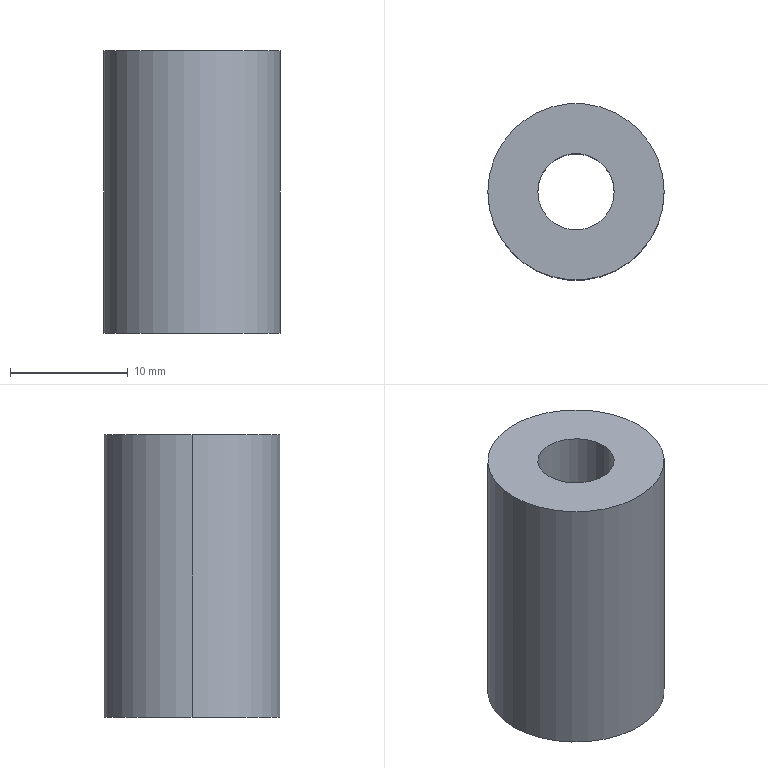Part | STEP file | track support post | 1 solid | 6 faces | box 15 x 15 x 24 mm | volume 3445 mm3 | cylinder 4 | plane 2 | commonest cylinder face diameters 6.5 x2 15 x2
STEP:
#1=CARTESIAN_POINT('',(0.,0.,0.));
#2=DIRECTION('',(0.,0.,1.));
#3=DIRECTION('',(1.,0.,0.));
#4=AXIS2_PLACEMENT_3D('',#1,#2,#3);
#5=CARTESIAN_POINT('',(3.25,0.,0.));
#6=VERTEX_POINT('',#5);
#7=CARTESIAN_POINT('',(3.25,0.,24.));
#8=VERTEX_POINT('',#7);
#9=CARTESIAN_POINT('',(3.25,0.,0.));
#10=DIRECTION('',(0.,0.,1.));
#11=VECTOR('',#10,1.);
#12=LINE('',#9,#11);
#13=CARTESIAN_POINT('',(0.,0.,0.));
#14=DIRECTION('',(0.,0.,1.));
#15=DIRECTION('',(1.,0.,0.));
#16=AXIS2_PLACEMENT_3D('',#13,#14,#15);
#17=CYLINDRICAL_SURFACE('',#16,3.25);
#18=CARTESIAN_POINT('',(6.283,0.));
#19=DIRECTION('',(0.,1.));
#20=VECTOR('',#19,1.);
#21=LINE('',#18,#20);
#22=(GEOMETRIC_REPRESENTATION_CONTEXT(2)PARAMETRIC_REPRESENTATION_CONTEXT()REPRESENTATION_CONTEXT('',''));
#23=DEFINITIONAL_REPRESENTATION('',(#21),#22);
#24=PCURVE('',#17,#23);
#25=CARTESIAN_POINT('',(0.,0.,0.));
#26=DIRECTION('',(0.,0.,1.));
#27=DIRECTION('',(1.,0.,0.));
#28=AXIS2_PLACEMENT_3D('',#25,#26,#27);
#29=CYLINDRICAL_SURFACE('',#28,3.25);
#30=CARTESIAN_POINT('',(0.,0.));
#31=DIRECTION('',(0.,1.));
#32=VECTOR('',#31,1.);
#33=LINE('',#30,#32);
#34=(GEOMETRIC_REPRESENTATION_CONTEXT(2)PARAMETRIC_REPRESENTATION_CONTEXT()REPRESENTATION_CONTEXT('',''));
#35=DEFINITIONAL_REPRESENTATION('',(#33),#34);
#36=PCURVE('',#29,#35);
#37=SURFACE_CURVE('',#12,(#24,#36),.PCURVE_S1.);
#38=EDGE_CURVE('',#6,#8,#37,.T.);
#39=ORIENTED_EDGE('',*,*,#38,.T.);
#40=CARTESIAN_POINT('',(-3.25,0.,24.));
#41=VERTEX_POINT('',#40);
#42=CARTESIAN_POINT('',(0.,0.,24.));
#43=DIRECTION('',(0.,0.,1.));
#44=DIRECTION('',(1.,0.,0.));
#45=AXIS2_PLACEMENT_3D('',#42,#43,#44);
#46=CIRCLE('',#45,3.25);
#47=CARTESIAN_POINT('',(0.,24.));
#48=DIRECTION('',(1.,0.));
#49=VECTOR('',#48,1.);
#50=LINE('',#47,#49);
#51=(GEOMETRIC_REPRESENTATION_CONTEXT(2)PARAMETRIC_REPRESENTATION_CONTEXT()REPRESENTATION_CONTEXT('',''));
#52=DEFINITIONAL_REPRESENTATION('',(#50),#51);
#53=PCURVE('',#17,#52);
#54=CARTESIAN_POINT('',(0.,0.,24.));
#55=DIRECTION('',(0.,0.,1.));
#56=DIRECTION('',(1.,0.,0.));
#57=AXIS2_PLACEMENT_3D('',#54,#55,#56);
#58=PLANE('',#57);
#59=CARTESIAN_POINT('',(0.,0.));
#60=DIRECTION('',(1.,0.));
#61=AXIS2_PLACEMENT_2D('',#59,#60);
#62=CIRCLE('',#61,3.25);
#63=(GEOMETRIC_REPRESENTATION_CONTEXT(2)PARAMETRIC_REPRESENTATION_CONTEXT()REPRESENTATION_CONTEXT('',''));
#64=DEFINITIONAL_REPRESENTATION('',(#62),#63);
#65=PCURVE('',#58,#64);
#66=SURFACE_CURVE('',#46,(#53,#65),.PCURVE_S1.);
#67=EDGE_CURVE('',#41,#8,#66,.T.);
#68=ORIENTED_EDGE('',*,*,#67,.F.);
#69=CARTESIAN_POINT('',(-3.25,0.,0.));
#70=VERTEX_POINT('',#69);
#71=CARTESIAN_POINT('',(-3.25,0.,0.));
#72=DIRECTION('',(0.,0.,1.));
#73=VECTOR('',#72,1.);
#74=LINE('',#71,#73);
#75=CARTESIAN_POINT('',(3.142,0.));
#76=DIRECTION('',(0.,1.));
#77=VECTOR('',#76,1.);
#78=LINE('',#75,#77);
#79=(GEOMETRIC_REPRESENTATION_CONTEXT(2)PARAMETRIC_REPRESENTATION_CONTEXT()REPRESENTATION_CONTEXT('',''));
#80=DEFINITIONAL_REPRESENTATION('',(#78),#79);
#81=PCURVE('',#17,#80);
#82=CARTESIAN_POINT('',(3.142,0.));
#83=DIRECTION('',(0.,1.));
#84=VECTOR('',#83,1.);
#85=LINE('',#82,#84);
#86=(GEOMETRIC_REPRESENTATION_CONTEXT(2)PARAMETRIC_REPRESENTATION_CONTEXT()REPRESENTATION_CONTEXT('',''));
#87=DEFINITIONAL_REPRESENTATION('',(#85),#86);
#88=PCURVE('',#29,#87);
#89=SURFACE_CURVE('',#74,(#81,#88),.PCURVE_S1.);
#90=EDGE_CURVE('',#70,#41,#89,.T.);
#91=ORIENTED_EDGE('',*,*,#90,.F.);
#92=CARTESIAN_POINT('',(0.,0.,0.));
#93=DIRECTION('',(0.,0.,1.));
#94=DIRECTION('',(1.,0.,0.));
#95=AXIS2_PLACEMENT_3D('',#92,#93,#94);
#96=CIRCLE('',#95,3.25);
#97=CARTESIAN_POINT('',(0.,0.));
#98=DIRECTION('',(1.,0.));
#99=VECTOR('',#98,1.);
#100=LINE('',#97,#99);
#101=(GEOMETRIC_REPRESENTATION_CONTEXT(2)PARAMETRIC_REPRESENTATION_CONTEXT()REPRESENTATION_CONTEXT('',''));
#102=DEFINITIONAL_REPRESENTATION('',(#100),#101);
#103=PCURVE('',#17,#102);
#104=CARTESIAN_POINT('',(0.,0.,0.));
#105=DIRECTION('',(0.,0.,1.));
#106=DIRECTION('',(1.,0.,0.));
#107=AXIS2_PLACEMENT_3D('',#104,#105,#106);
#108=PLANE('',#107);
#109=CARTESIAN_POINT('',(0.,0.));
#110=DIRECTION('',(1.,0.));
#111=AXIS2_PLACEMENT_2D('',#109,#110);
#112=CIRCLE('',#111,3.25);
#113=(GEOMETRIC_REPRESENTATION_CONTEXT(2)PARAMETRIC_REPRESENTATION_CONTEXT()REPRESENTATION_CONTEXT('',''));
#114=DEFINITIONAL_REPRESENTATION('',(#112),#113);
#115=PCURVE('',#108,#114);
#116=SURFACE_CURVE('',#96,(#103,#115),.PCURVE_S1.);
#117=EDGE_CURVE('',#70,#6,#116,.T.);
#118=ORIENTED_EDGE('',*,*,#117,.T.);
#119=EDGE_LOOP('',(#39,#68,#91,#118));
#120=FACE_BOUND('',#119,.F.);
#121=ADVANCED_FACE('',(#120),#17,.F.);
#122=CARTESIAN_POINT('',(7.5,0.,24.));
#123=VERTEX_POINT('',#122);
#124=CARTESIAN_POINT('',(-7.5,0.,24.));
#125=VERTEX_POINT('',#124);
#126=CARTESIAN_POINT('',(0.,0.,24.));
#127=DIRECTION('',(0.,0.,1.));
#128=DIRECTION('',(1.,0.,0.));
#129=AXIS2_PLACEMENT_3D('',#126,#127,#128);
#130=CIRCLE('',#129,7.5);
#131=CARTESIAN_POINT('',(0.,0.,24.));
#132=DIRECTION('',(0.,0.,-1.));
#133=DIRECTION('',(-1.,0.,0.));
#134=AXIS2_PLACEMENT_3D('',#131,#132,#133);
#135=CYLINDRICAL_SURFACE('',#134,7.5);
#136=CARTESIAN_POINT('',(3.142,0.));
#137=DIRECTION('',(-1.,0.));
#138=VECTOR('',#137,1.);
#139=LINE('',#136,#138);
#140=(GEOMETRIC_REPRESENTATION_CONTEXT(2)PARAMETRIC_REPRESENTATION_CONTEXT()REPRESENTATION_CONTEXT('',''));
#141=DEFINITIONAL_REPRESENTATION('',(#139),#140);
#142=PCURVE('',#135,#141);
#143=CARTESIAN_POINT('',(0.,0.));
#144=DIRECTION('',(1.,0.));
#145=AXIS2_PLACEMENT_2D('',#143,#144);
#146=CIRCLE('',#145,7.5);
#147=(GEOMETRIC_REPRESENTATION_CONTEXT(2)PARAMETRIC_REPRESENTATION_CONTEXT()REPRESENTATION_CONTEXT('',''));
#148=DEFINITIONAL_REPRESENTATION('',(#146),#147);
#149=PCURVE('',#58,#148);
#150=SURFACE_CURVE('',#130,(#142,#149),.PCURVE_S1.);
#151=EDGE_CURVE('',#123,#125,#150,.T.);
#152=ORIENTED_EDGE('',*,*,#151,.F.);
#153=CARTESIAN_POINT('',(7.5,0.,0.));
#154=VERTEX_POINT('',#153);
#155=CARTESIAN_POINT('',(7.5,0.,24.));
#156=DIRECTION('',(0.,0.,-1.));
#157=VECTOR('',#156,1.);
#158=LINE('',#155,#157);
#159=CARTESIAN_POINT('',(3.142,0.));
#160=DIRECTION('',(0.,1.));
#161=VECTOR('',#160,1.);
#162=LINE('',#159,#161);
#163=(GEOMETRIC_REPRESENTATION_CONTEXT(2)PARAMETRIC_REPRESENTATION_CONTEXT()REPRESENTATION_CONTEXT('',''));
#164=DEFINITIONAL_REPRESENTATION('',(#162),#163);
#165=PCURVE('',#135,#164);
#166=CARTESIAN_POINT('',(0.,0.,24.));
#167=DIRECTION('',(0.,0.,-1.));
#168=DIRECTION('',(-1.,0.,0.));
#169=AXIS2_PLACEMENT_3D('',#166,#167,#168);
#170=CYLINDRICAL_SURFACE('',#169,7.5);
#171=CARTESIAN_POINT('',(3.142,0.));
#172=DIRECTION('',(0.,1.));
#173=VECTOR('',#172,1.);
#174=LINE('',#171,#173);
#175=(GEOMETRIC_REPRESENTATION_CONTEXT(2)PARAMETRIC_REPRESENTATION_CONTEXT()REPRESENTATION_CONTEXT('',''));
#176=DEFINITIONAL_REPRESENTATION('',(#174),#175);
#177=PCURVE('',#170,#176);
#178=SURFACE_CURVE('',#158,(#165,#177),.PCURVE_S1.);
#179=EDGE_CURVE('',#123,#154,#178,.T.);
#180=ORIENTED_EDGE('',*,*,#179,.T.);
#181=CARTESIAN_POINT('',(-7.5,0.,0.));
#182=VERTEX_POINT('',#181);
#183=CARTESIAN_POINT('',(0.,0.,0.));
#184=DIRECTION('',(0.,0.,1.));
#185=DIRECTION('',(1.,0.,0.));
#186=AXIS2_PLACEMENT_3D('',#183,#184,#185);
#187=CIRCLE('',#186,7.5);
#188=CARTESIAN_POINT('',(3.142,24.));
#189=DIRECTION('',(-1.,0.));
#190=VECTOR('',#189,1.);
#191=LINE('',#188,#190);
#192=(GEOMETRIC_REPRESENTATION_CONTEXT(2)PARAMETRIC_REPRESENTATION_CONTEXT()REPRESENTATION_CONTEXT('',''));
#193=DEFINITIONAL_REPRESENTATION('',(#191),#192);
#194=PCURVE('',#135,#193);
#195=CARTESIAN_POINT('',(0.,0.));
#196=DIRECTION('',(1.,0.));
#197=AXIS2_PLACEMENT_2D('',#195,#196);
#198=CIRCLE('',#197,7.5);
#199=(GEOMETRIC_REPRESENTATION_CONTEXT(2)PARAMETRIC_REPRESENTATION_CONTEXT()REPRESENTATION_CONTEXT('',''));
#200=DEFINITIONAL_REPRESENTATION('',(#198),#199);
#201=PCURVE('',#108,#200);
#202=SURFACE_CURVE('',#187,(#194,#201),.PCURVE_S1.);
#203=EDGE_CURVE('',#154,#182,#202,.T.);
#204=ORIENTED_EDGE('',*,*,#203,.T.);
#205=CARTESIAN_POINT('',(-7.5,0.,24.));
#206=DIRECTION('',(0.,0.,-1.));
#207=VECTOR('',#206,1.);
#208=LINE('',#205,#207);
#209=CARTESIAN_POINT('',(0.,0.));
#210=DIRECTION('',(0.,1.));
#211=VECTOR('',#210,1.);
#212=LINE('',#209,#211);
#213=(GEOMETRIC_REPRESENTATION_CONTEXT(2)PARAMETRIC_REPRESENTATION_CONTEXT()REPRESENTATION_CONTEXT('',''));
#214=DEFINITIONAL_REPRESENTATION('',(#212),#213);
#215=PCURVE('',#135,#214);
#216=CARTESIAN_POINT('',(6.283,0.));
#217=DIRECTION('',(0.,1.));
#218=VECTOR('',#217,1.);
#219=LINE('',#216,#218);
#220=(GEOMETRIC_REPRESENTATION_CONTEXT(2)PARAMETRIC_REPRESENTATION_CONTEXT()REPRESENTATION_CONTEXT('',''));
#221=DEFINITIONAL_REPRESENTATION('',(#219),#220);
#222=PCURVE('',#170,#221);
#223=SURFACE_CURVE('',#208,(#215,#222),.PCURVE_S1.);
#224=EDGE_CURVE('',#125,#182,#223,.T.);
#225=ORIENTED_EDGE('',*,*,#224,.F.);
#226=EDGE_LOOP('',(#152,#180,#204,#225));
#227=FACE_BOUND('',#226,.T.);
#228=ADVANCED_FACE('',(#227),#135,.T.);
#229=ORIENTED_EDGE('',*,*,#179,.F.);
#230=CARTESIAN_POINT('',(0.,0.,24.));
#231=DIRECTION('',(0.,0.,1.));
#232=DIRECTION('',(1.,0.,0.));
#233=AXIS2_PLACEMENT_3D('',#230,#231,#232);
#234=CIRCLE('',#233,7.5);
#235=CARTESIAN_POINT('',(9.425,0.));
#236=DIRECTION('',(-1.,0.));
#237=VECTOR('',#236,1.);
#238=LINE('',#235,#237);
#239=(GEOMETRIC_REPRESENTATION_CONTEXT(2)PARAMETRIC_REPRESENTATION_CONTEXT()REPRESENTATION_CONTEXT('',''));
#240=DEFINITIONAL_REPRESENTATION('',(#238),#239);
#241=PCURVE('',#170,#240);
#242=CARTESIAN_POINT('',(0.,0.));
#243=DIRECTION('',(1.,0.));
#244=AXIS2_PLACEMENT_2D('',#242,#243);
#245=CIRCLE('',#244,7.5);
#246=(GEOMETRIC_REPRESENTATION_CONTEXT(2)PARAMETRIC_REPRESENTATION_CONTEXT()REPRESENTATION_CONTEXT('',''));
#247=DEFINITIONAL_REPRESENTATION('',(#245),#246);
#248=PCURVE('',#58,#247);
#249=SURFACE_CURVE('',#234,(#241,#248),.PCURVE_S1.);
#250=EDGE_CURVE('',#125,#123,#249,.T.);
#251=ORIENTED_EDGE('',*,*,#250,.F.);
#252=ORIENTED_EDGE('',*,*,#224,.T.);
#253=CARTESIAN_POINT('',(0.,0.,0.));
#254=DIRECTION('',(0.,0.,1.));
#255=DIRECTION('',(1.,0.,0.));
#256=AXIS2_PLACEMENT_3D('',#253,#254,#255);
#257=CIRCLE('',#256,7.5);
#258=CARTESIAN_POINT('',(9.425,24.));
#259=DIRECTION('',(-1.,0.));
#260=VECTOR('',#259,1.);
#261=LINE('',#258,#260);
#262=(GEOMETRIC_REPRESENTATION_CONTEXT(2)PARAMETRIC_REPRESENTATION_CONTEXT()REPRESENTATION_CONTEXT('',''));
#263=DEFINITIONAL_REPRESENTATION('',(#261),#262);
#264=PCURVE('',#170,#263);
#265=CARTESIAN_POINT('',(0.,0.));
#266=DIRECTION('',(1.,0.));
#267=AXIS2_PLACEMENT_2D('',#265,#266);
#268=CIRCLE('',#267,7.5);
#269=(GEOMETRIC_REPRESENTATION_CONTEXT(2)PARAMETRIC_REPRESENTATION_CONTEXT()REPRESENTATION_CONTEXT('',''));
#270=DEFINITIONAL_REPRESENTATION('',(#268),#269);
#271=PCURVE('',#108,#270);
#272=SURFACE_CURVE('',#257,(#264,#271),.PCURVE_S1.);
#273=EDGE_CURVE('',#182,#154,#272,.T.);
#274=ORIENTED_EDGE('',*,*,#273,.T.);
#275=EDGE_LOOP('',(#229,#251,#252,#274));
#276=FACE_BOUND('',#275,.T.);
#277=ADVANCED_FACE('',(#276),#170,.T.);
#278=CARTESIAN_POINT('',(0.,0.,24.));
#279=DIRECTION('',(0.,0.,1.));
#280=DIRECTION('',(1.,0.,0.));
#281=AXIS2_PLACEMENT_3D('',#278,#279,#280);
#282=CIRCLE('',#281,3.25);
#283=CARTESIAN_POINT('',(0.,0.));
#284=DIRECTION('',(1.,0.));
#285=AXIS2_PLACEMENT_2D('',#283,#284);
#286=CIRCLE('',#285,3.25);
#287=(GEOMETRIC_REPRESENTATION_CONTEXT(2)PARAMETRIC_REPRESENTATION_CONTEXT()REPRESENTATION_CONTEXT('',''));
#288=DEFINITIONAL_REPRESENTATION('',(#286),#287);
#289=PCURVE('',#58,#288);
#290=CARTESIAN_POINT('',(0.,24.));
#291=DIRECTION('',(1.,0.));
#292=VECTOR('',#291,1.);
#293=LINE('',#290,#292);
#294=(GEOMETRIC_REPRESENTATION_CONTEXT(2)PARAMETRIC_REPRESENTATION_CONTEXT()REPRESENTATION_CONTEXT('',''));
#295=DEFINITIONAL_REPRESENTATION('',(#293),#294);
#296=PCURVE('',#29,#295);
#297=SURFACE_CURVE('',#282,(#289,#296),.PCURVE_S1.);
#298=EDGE_CURVE('',#8,#41,#297,.T.);
#299=ORIENTED_EDGE('',*,*,#298,.F.);
#300=ORIENTED_EDGE('',*,*,#67,.F.);
#301=EDGE_LOOP('',(#299,#300));
#302=FACE_BOUND('',#301,.T.);
#303=ORIENTED_EDGE('',*,*,#250,.T.);
#304=ORIENTED_EDGE('',*,*,#151,.T.);
#305=EDGE_LOOP('',(#303,#304));
#306=FACE_BOUND('',#305,.T.);
#307=ADVANCED_FACE('',(#302,#306),#58,.T.);
#308=CARTESIAN_POINT('',(0.,0.,0.));
#309=DIRECTION('',(0.,0.,1.));
#310=DIRECTION('',(1.,0.,0.));
#311=AXIS2_PLACEMENT_3D('',#308,#309,#310);
#312=CIRCLE('',#311,3.25);
#313=CARTESIAN_POINT('',(0.,0.));
#314=DIRECTION('',(1.,0.));
#315=AXIS2_PLACEMENT_2D('',#313,#314);
#316=CIRCLE('',#315,3.25);
#317=(GEOMETRIC_REPRESENTATION_CONTEXT(2)PARAMETRIC_REPRESENTATION_CONTEXT()REPRESENTATION_CONTEXT('',''));
#318=DEFINITIONAL_REPRESENTATION('',(#316),#317);
#319=PCURVE('',#108,#318);
#320=CARTESIAN_POINT('',(0.,0.));
#321=DIRECTION('',(1.,0.));
#322=VECTOR('',#321,1.);
#323=LINE('',#320,#322);
#324=(GEOMETRIC_REPRESENTATION_CONTEXT(2)PARAMETRIC_REPRESENTATION_CONTEXT()REPRESENTATION_CONTEXT('',''));
#325=DEFINITIONAL_REPRESENTATION('',(#323),#324);
#326=PCURVE('',#29,#325);
#327=SURFACE_CURVE('',#312,(#319,#326),.PCURVE_S1.);
#328=EDGE_CURVE('',#6,#70,#327,.T.);
#329=ORIENTED_EDGE('',*,*,#328,.T.);
#330=ORIENTED_EDGE('',*,*,#117,.T.);
#331=EDGE_LOOP('',(#329,#330));
#332=FACE_BOUND('',#331,.T.);
#333=ORIENTED_EDGE('',*,*,#273,.F.);
#334=ORIENTED_EDGE('',*,*,#203,.F.);
#335=EDGE_LOOP('',(#333,#334));
#336=FACE_BOUND('',#335,.T.);
#337=ADVANCED_FACE('',(#332,#336),#108,.F.);
#338=ORIENTED_EDGE('',*,*,#298,.F.);
#339=ORIENTED_EDGE('',*,*,#38,.F.);
#340=ORIENTED_EDGE('',*,*,#328,.T.);
#341=ORIENTED_EDGE('',*,*,#90,.T.);
#342=EDGE_LOOP('',(#338,#339,#340,#341));
#343=FACE_BOUND('',#342,.F.);
#344=ADVANCED_FACE('',(#343),#29,.F.);
#345=CLOSED_SHELL('',(#121,#228,#277,#307,#337,#344));
#346=MANIFOLD_SOLID_BREP('',#345);
#347=(LENGTH_UNIT()NAMED_UNIT(*)SI_UNIT(.MILLI.,.METRE.));
#348=UNCERTAINTY_MEASURE_WITH_UNIT(LENGTH_MEASURE(0.0000001),#347,'','');
#349=(NAMED_UNIT(*)PLANE_ANGLE_UNIT()SI_UNIT($,.RADIAN.));
#350=(NAMED_UNIT(*)SI_UNIT($,.STERADIAN.)SOLID_ANGLE_UNIT());
#351=(GEOMETRIC_REPRESENTATION_CONTEXT(3)GLOBAL_UNCERTAINTY_ASSIGNED_CONTEXT((#348))GLOBAL_UNIT_ASSIGNED_CONTEXT((#347,#349,#350))REPRESENTATION_CONTEXT('',''));
#352=ADVANCED_BREP_SHAPE_REPRESENTATION('',(#4,#346),#351);